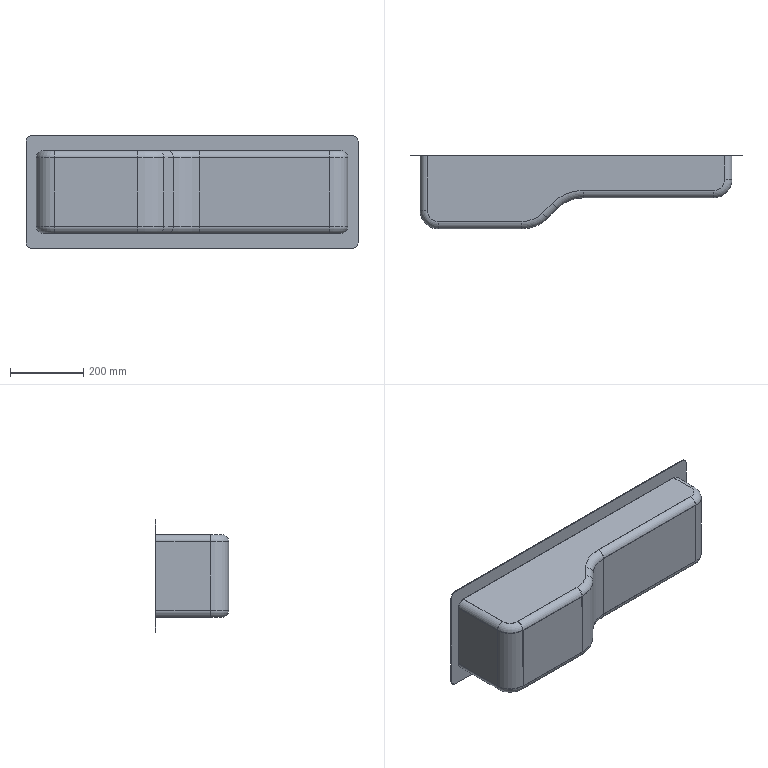Part | SolidWorks | features BaseBody 2 | 2 solids | 77 faces | box 908 x 201.5 x 308 mm | volume 869996 mm3 | cylinder 36 | plane 25 | torus 16 | commonest cylinder face diameters 40 x14 37 x10 30 x4 97 x2 100 x2 200 x2